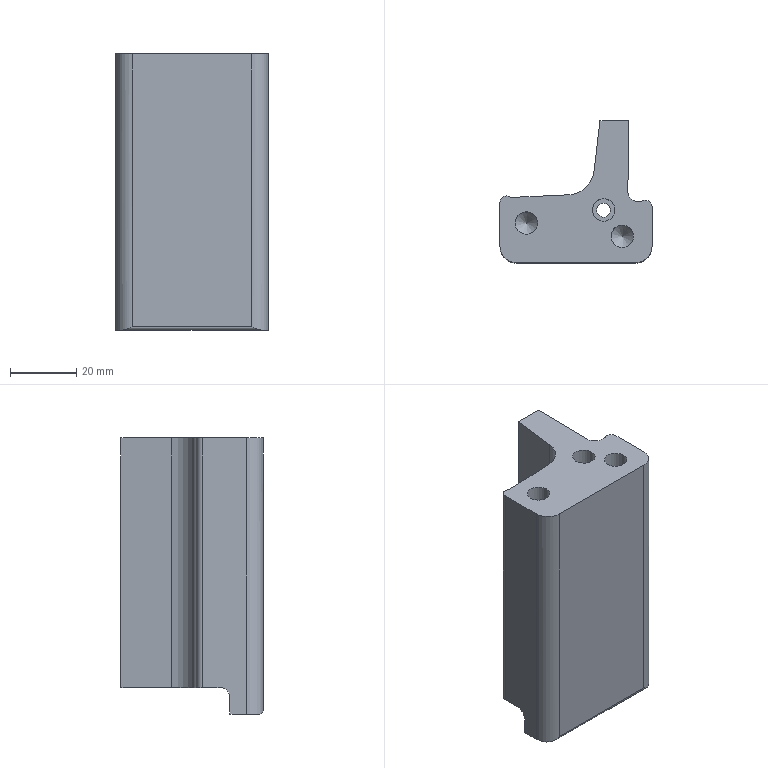Part | NX | features solid 2 | 1 solid | 32 faces | box 46 x 42.956 x 83.5 mm | volume 85744 mm3 | cylinder 15 | plane 14 | cone 3 | commonest cylinder face diameters 4 x4 6.8 x3 6 x2 10 x2 2 x1 4.2 x1
STEP:
#1=CARTESIAN_POINT('',(81.,-103.,-13.5));
#2=VERTEX_POINT('',#1);
#3=CARTESIAN_POINT('',(79.,-107.,-13.5));
#4=VERTEX_POINT('',#3);
#5=CARTESIAN_POINT('',(76.,-103.,-13.5));
#6=DIRECTION('',(0.,0.,-1.));
#7=DIRECTION('',(-1.,0.,0.));
#8=AXIS2_PLACEMENT_3D('',#5,#6,#7);
#9=CIRCLE('',#8,5.);
#10=EDGE_CURVE('',#2,#4,#9,.T.);
#11=ORIENTED_EDGE('',*,*,#10,.T.);
#12=CARTESIAN_POINT('',(37.,-107.,-13.5));
#13=VERTEX_POINT('',#12);
#14=CARTESIAN_POINT('',(16.212,-107.,-13.5));
#15=DIRECTION('',(-1.,0.,0.));
#16=VECTOR('',#15,1000.);
#17=LINE('',#14,#16);
#18=EDGE_CURVE('',#4,#13,#17,.T.);
#19=ORIENTED_EDGE('',*,*,#18,.T.);
#20=CARTESIAN_POINT('',(35.,-103.,-13.5));
#21=VERTEX_POINT('',#20);
#22=CARTESIAN_POINT('',(40.,-103.,-13.5));
#23=DIRECTION('',(0.,0.,-1.));
#24=DIRECTION('',(-1.,0.,0.));
#25=AXIS2_PLACEMENT_3D('',#22,#23,#24);
#26=CIRCLE('',#25,5.);
#27=EDGE_CURVE('',#13,#21,#26,.T.);
#28=ORIENTED_EDGE('',*,*,#27,.T.);
#29=CARTESIAN_POINT('',(35.,-98.,-13.5));
#30=VERTEX_POINT('',#29);
#31=CARTESIAN_POINT('',(35.,-108.,-13.5));
#32=DIRECTION('',(0.,1.,0.));
#33=VECTOR('',#32,1000.);
#34=LINE('',#31,#33);
#35=EDGE_CURVE('',#21,#30,#34,.T.);
#36=ORIENTED_EDGE('',*,*,#35,.T.);
#37=CARTESIAN_POINT('',(81.,-98.,-13.5));
#38=VERTEX_POINT('',#37);
#39=CARTESIAN_POINT('',(16.212,-98.,-13.5));
#40=DIRECTION('',(-1.,0.,0.));
#41=VECTOR('',#40,1000.);
#42=LINE('',#39,#41);
#43=EDGE_CURVE('',#38,#30,#42,.T.);
#44=ORIENTED_EDGE('',*,*,#43,.F.);
#45=CARTESIAN_POINT('',(81.,-108.,-13.5));
#46=DIRECTION('',(0.,1.,0.));
#47=VECTOR('',#46,1000.);
#48=LINE('',#45,#47);
#49=EDGE_CURVE('',#2,#38,#48,.T.);
#50=ORIENTED_EDGE('',*,*,#49,.F.);
#51=EDGE_LOOP('',(#11,#19,#28,#36,#44,#50));
#52=FACE_BOUND('',#51,.T.);
#53=CARTESIAN_POINT('',(55.4,-103.,-13.5));
#54=VERTEX_POINT('',#53);
#55=CARTESIAN_POINT('',(58.,-103.,-13.5));
#56=DIRECTION('',(0.,0.,-1.));
#57=DIRECTION('',(-1.,0.,0.));
#58=AXIS2_PLACEMENT_3D('',#55,#56,#57);
#59=CIRCLE('',#58,2.6);
#60=EDGE_CURVE('',#54,#54,#59,.F.);
#61=ORIENTED_EDGE('',*,*,#60,.T.);
#62=EDGE_LOOP('',(#61));
#63=FACE_BOUND('',#62,.T.);
#64=CARTESIAN_POINT('',(16.212,-108.,-13.5));
#65=DIRECTION('',(0.,0.,-1.));
#66=DIRECTION('',(-1.,0.,0.));
#67=AXIS2_PLACEMENT_3D('',#64,#65,#66);
#68=PLANE('',#67);
#69=ADVANCED_FACE('',(#52,#63),#68,.T.);
#70=CARTESIAN_POINT('',(46.4,-96.,70.));
#71=VERTEX_POINT('',#70);
#72=CARTESIAN_POINT('',(43.,-96.,70.));
#73=DIRECTION('',(0.,0.,-1.));
#74=DIRECTION('',(1.,0.,0.));
#75=AXIS2_PLACEMENT_3D('',#72,#73,#74);
#76=CIRCLE('',#75,3.4);
#77=EDGE_CURVE('',#71,#71,#76,.T.);
#78=ORIENTED_EDGE('',*,*,#77,.T.);
#79=EDGE_LOOP('',(#78));
#80=FACE_BOUND('',#79,.T.);
#81=CARTESIAN_POINT('',(69.763,-92.,70.));
#82=VERTEX_POINT('',#81);
#83=CARTESIAN_POINT('',(66.363,-92.,70.));
#84=DIRECTION('',(0.,0.,1.));
#85=DIRECTION('',(1.,0.,0.));
#86=AXIS2_PLACEMENT_3D('',#83,#84,#85);
#87=CIRCLE('',#86,3.4);
#88=EDGE_CURVE('',#82,#82,#87,.T.);
#89=ORIENTED_EDGE('',*,*,#88,.F.);
#90=EDGE_LOOP('',(#89));
#91=FACE_BOUND('',#90,.T.);
#92=CARTESIAN_POINT('',(73.954,-65.044,70.));
#93=VERTEX_POINT('',#92);
#94=CARTESIAN_POINT('',(73.682,-86.43,70.));
#95=VERTEX_POINT('',#94);
#96=CARTESIAN_POINT('',(74.016,-60.221,70.));
#97=DIRECTION('',(-0.01273,-0.9999,0.));
#98=VECTOR('',#97,1000.);
#99=LINE('',#96,#98);
#100=EDGE_CURVE('',#93,#95,#99,.T.);
#101=ORIENTED_EDGE('',*,*,#100,.F.);
#102=CARTESIAN_POINT('',(65.247,-65.044,70.));
#103=VERTEX_POINT('',#102);
#104=CARTESIAN_POINT('',(-37.5,-65.044,70.));
#105=DIRECTION('',(-1.,0.,0.));
#106=VECTOR('',#105,1000.);
#107=LINE('',#104,#106);
#108=EDGE_CURVE('',#103,#93,#107,.F.);
#109=ORIENTED_EDGE('',*,*,#108,.F.);
#110=CARTESIAN_POINT('',(63.441,-80.376,70.));
#111=VERTEX_POINT('',#110);
#112=CARTESIAN_POINT('',(63.441,-80.376,70.));
#113=DIRECTION('',(0.117,0.9931,0.));
#114=VECTOR('',#113,1000.);
#115=LINE('',#112,#114);
#116=EDGE_CURVE('',#103,#111,#115,.F.);
#117=ORIENTED_EDGE('',*,*,#116,.T.);
#118=CARTESIAN_POINT('',(55.874,-87.431,70.));
#119=VERTEX_POINT('',#118);
#120=CARTESIAN_POINT('',(55.496,-79.44,70.));
#121=DIRECTION('',(0.,0.,1.));
#122=DIRECTION('',(1.,0.,0.));
#123=AXIS2_PLACEMENT_3D('',#120,#121,#122);
#124=CIRCLE('',#123,8.);
#125=EDGE_CURVE('',#111,#119,#124,.F.);
#126=ORIENTED_EDGE('',*,*,#125,.T.);
#127=CARTESIAN_POINT('',(46.55,-87.872,70.));
#128=VERTEX_POINT('',#127);
#129=CARTESIAN_POINT('',(46.55,-87.872,70.));
#130=DIRECTION('',(0.9989,0.04722,0.));
#131=VECTOR('',#130,1000.);
#132=LINE('',#129,#131);
#133=EDGE_CURVE('',#119,#128,#132,.F.);
#134=ORIENTED_EDGE('',*,*,#133,.T.);
#135=CARTESIAN_POINT('',(38.87,-88.202,70.));
#136=VERTEX_POINT('',#135);
#137=CARTESIAN_POINT('',(38.87,-88.202,70.));
#138=DIRECTION('',(0.9991,0.0429,0.));
#139=VECTOR('',#138,1000.);
#140=LINE('',#137,#139);
#141=EDGE_CURVE('',#136,#128,#140,.T.);
#142=ORIENTED_EDGE('',*,*,#141,.F.);
#143=CARTESIAN_POINT('',(37.892,-87.994,70.));
#144=VERTEX_POINT('',#143);
#145=CARTESIAN_POINT('',(38.784,-86.203,70.));
#146=DIRECTION('',(0.,0.,1.));
#147=DIRECTION('',(1.,0.,0.));
#148=AXIS2_PLACEMENT_3D('',#145,#146,#147);
#149=CIRCLE('',#148,2.);
#150=EDGE_CURVE('',#144,#136,#149,.T.);
#151=ORIENTED_EDGE('',*,*,#150,.F.);
#152=CARTESIAN_POINT('',(35.,-89.784,70.));
#153=VERTEX_POINT('',#152);
#154=CARTESIAN_POINT('',(37.,-89.784,70.));
#155=DIRECTION('',(0.,0.,1.));
#156=DIRECTION('',(1.,0.,0.));
#157=AXIS2_PLACEMENT_3D('',#154,#155,#156);
#158=CIRCLE('',#157,2.);
#159=EDGE_CURVE('',#153,#144,#158,.F.);
#160=ORIENTED_EDGE('',*,*,#159,.F.);
#161=CARTESIAN_POINT('',(35.,-103.,70.));
#162=VERTEX_POINT('',#161);
#163=CARTESIAN_POINT('',(35.,-110.403,70.));
#164=DIRECTION('',(0.,1.,0.));
#165=VECTOR('',#164,1000.);
#166=LINE('',#163,#165);
#167=EDGE_CURVE('',#162,#153,#166,.T.);
#168=ORIENTED_EDGE('',*,*,#167,.F.);
#169=CARTESIAN_POINT('',(40.,-108.,70.));
#170=VERTEX_POINT('',#169);
#171=CARTESIAN_POINT('',(40.,-103.,70.));
#172=DIRECTION('',(0.,0.,1.));
#173=DIRECTION('',(1.,0.,0.));
#174=AXIS2_PLACEMENT_3D('',#171,#172,#173);
#175=CIRCLE('',#174,5.);
#176=EDGE_CURVE('',#170,#162,#175,.F.);
#177=ORIENTED_EDGE('',*,*,#176,.F.);
#178=CARTESIAN_POINT('',(76.,-108.,70.));
#179=VERTEX_POINT('',#178);
#180=CARTESIAN_POINT('',(16.212,-108.,70.));
#181=DIRECTION('',(-1.,0.,0.));
#182=VECTOR('',#181,1000.);
#183=LINE('',#180,#182);
#184=EDGE_CURVE('',#179,#170,#183,.T.);
#185=ORIENTED_EDGE('',*,*,#184,.F.);
#186=CARTESIAN_POINT('',(81.,-103.,70.));
#187=VERTEX_POINT('',#186);
#188=CARTESIAN_POINT('',(76.,-103.,70.));
#189=DIRECTION('',(0.,0.,1.));
#190=DIRECTION('',(1.,0.,0.));
#191=AXIS2_PLACEMENT_3D('',#188,#189,#190);
#192=CIRCLE('',#191,5.);
#193=EDGE_CURVE('',#187,#179,#192,.F.);
#194=ORIENTED_EDGE('',*,*,#193,.F.);
#195=CARTESIAN_POINT('',(81.,-91.098,70.));
#196=VERTEX_POINT('',#195);
#197=CARTESIAN_POINT('',(81.,-91.098,70.));
#198=DIRECTION('',(0.,-1.,0.));
#199=VECTOR('',#198,1000.);
#200=LINE('',#197,#199);
#201=EDGE_CURVE('',#196,#187,#200,.T.);
#202=ORIENTED_EDGE('',*,*,#201,.F.);
#203=CARTESIAN_POINT('',(78.127,-89.299,70.));
#204=VERTEX_POINT('',#203);
#205=CARTESIAN_POINT('',(79.,-91.098,70.));
#206=DIRECTION('',(0.,0.,1.));
#207=DIRECTION('',(1.,0.,0.));
#208=AXIS2_PLACEMENT_3D('',#205,#206,#207);
#209=CIRCLE('',#208,2.);
#210=EDGE_CURVE('',#204,#196,#209,.F.);
#211=ORIENTED_EDGE('',*,*,#210,.F.);
#212=CARTESIAN_POINT('',(77.147,-89.497,70.));
#213=VERTEX_POINT('',#212);
#214=CARTESIAN_POINT('',(77.253,-87.5,70.));
#215=DIRECTION('',(0.,0.,1.));
#216=DIRECTION('',(1.,0.,0.));
#217=AXIS2_PLACEMENT_3D('',#214,#215,#216);
#218=CIRCLE('',#217,2.);
#219=EDGE_CURVE('',#213,#204,#218,.T.);
#220=ORIENTED_EDGE('',*,*,#219,.F.);
#221=CARTESIAN_POINT('',(76.523,-89.464,70.));
#222=VERTEX_POINT('',#221);
#223=CARTESIAN_POINT('',(76.523,-89.464,70.));
#224=DIRECTION('',(0.9986,-0.05307,0.));
#225=VECTOR('',#224,1000.);
#226=LINE('',#223,#225);
#227=EDGE_CURVE('',#222,#213,#226,.T.);
#228=ORIENTED_EDGE('',*,*,#227,.F.);
#229=CARTESIAN_POINT('',(76.682,-86.468,70.));
#230=DIRECTION('',(0.,0.,1.));
#231=DIRECTION('',(1.,0.,0.));
#232=AXIS2_PLACEMENT_3D('',#229,#230,#231);
#233=CIRCLE('',#232,3.);
#234=EDGE_CURVE('',#95,#222,#233,.T.);
#235=ORIENTED_EDGE('',*,*,#234,.F.);
#236=EDGE_LOOP('',(#101,#109,#117,#126,#134,#142,#151,#160,#168,#177,#185,#194,#202,#211,#220,#228,#235));
#237=FACE_BOUND('',#236,.T.);
#238=CARTESIAN_POINT('',(75.4,-100.,70.));
#239=VERTEX_POINT('',#238);
#240=CARTESIAN_POINT('',(72.,-100.,70.));
#241=DIRECTION('',(0.,0.,-1.));
#242=DIRECTION('',(1.,0.,0.));
#243=AXIS2_PLACEMENT_3D('',#240,#241,#242);
#244=CIRCLE('',#243,3.4);
#245=EDGE_CURVE('',#239,#239,#244,.T.);
#246=ORIENTED_EDGE('',*,*,#245,.T.);
#247=EDGE_LOOP('',(#246));
#248=FACE_BOUND('',#247,.T.);
#249=CARTESIAN_POINT('',(-37.5,0.,70.));
#250=DIRECTION('',(0.,0.,1.));
#251=DIRECTION('',(1.,0.,0.));
#252=AXIS2_PLACEMENT_3D('',#249,#250,#251);
#253=PLANE('',#252);
#254=ADVANCED_FACE('',(#80,#91,#237,#248),#253,.T.);
#255=CARTESIAN_POINT('',(76.,-108.,-12.5));
#256=VERTEX_POINT('',#255);
#257=CARTESIAN_POINT('',(79.,-107.,-13.5));
#258=CARTESIAN_POINT('',(78.085,-107.686,-13.5));
#259=CARTESIAN_POINT('',(77.03,-108.,-12.961));
#260=CARTESIAN_POINT('',(76.,-108.,-12.5));
#261=B_SPLINE_CURVE_WITH_KNOTS('',3,(#257,#258,#259,#260),.UNSPECIFIED.,.F.,.F.,(4,4),(0.,0.003386),.UNSPECIFIED.);
#262=EDGE_CURVE('',#256,#4,#261,.F.);
#263=ORIENTED_EDGE('',*,*,#262,.F.);
#264=CARTESIAN_POINT('',(40.,-108.,-12.5));
#265=VERTEX_POINT('',#264);
#266=CARTESIAN_POINT('',(16.212,-108.,-12.5));
#267=DIRECTION('',(-1.,0.,0.));
#268=VECTOR('',#267,1000.);
#269=LINE('',#266,#268);
#270=EDGE_CURVE('',#265,#256,#269,.F.);
#271=ORIENTED_EDGE('',*,*,#270,.F.);
#272=CARTESIAN_POINT('',(37.,-107.,-13.5));
#273=CARTESIAN_POINT('',(37.915,-107.686,-13.5));
#274=CARTESIAN_POINT('',(38.97,-108.,-12.961));
#275=CARTESIAN_POINT('',(40.,-108.,-12.5));
#276=B_SPLINE_CURVE_WITH_KNOTS('',3,(#272,#273,#274,#275),.UNSPECIFIED.,.F.,.F.,(4,4),(0.,0.003386),.UNSPECIFIED.);
#277=EDGE_CURVE('',#13,#265,#276,.T.);
#278=ORIENTED_EDGE('',*,*,#277,.F.);
#279=ORIENTED_EDGE('',*,*,#18,.F.);
#280=EDGE_LOOP('',(#263,#271,#278,#279));
#281=FACE_BOUND('',#280,.T.);
#282=CARTESIAN_POINT('',(16.212,-107.,-12.5));
#283=DIRECTION('',(-1.,0.,0.));
#284=DIRECTION('',(0.,0.,1.));
#285=AXIS2_PLACEMENT_3D('',#282,#283,#284);
#286=CYLINDRICAL_SURFACE('',#285,1.);
#287=ADVANCED_FACE('',(#281),#286,.T.);
#288=CARTESIAN_POINT('',(35.,-98.,-8.5));
#289=VERTEX_POINT('',#288);
#290=CARTESIAN_POINT('',(35.,-98.,40.));
#291=DIRECTION('',(0.,0.,-1.));
#292=VECTOR('',#291,1000.);
#293=LINE('',#290,#292);
#294=EDGE_CURVE('',#289,#30,#293,.T.);
#295=ORIENTED_EDGE('',*,*,#294,.F.);
#296=CARTESIAN_POINT('',(81.,-98.,-8.5));
#297=VERTEX_POINT('',#296);
#298=CARTESIAN_POINT('',(81.,-98.,-8.5));
#299=DIRECTION('',(-1.,0.,0.));
#300=VECTOR('',#299,1000.);
#301=LINE('',#298,#300);
#302=EDGE_CURVE('',#289,#297,#301,.F.);
#303=ORIENTED_EDGE('',*,*,#302,.T.);
#304=CARTESIAN_POINT('',(81.,-98.,40.));
#305=DIRECTION('',(0.,0.,-1.));
#306=VECTOR('',#305,1000.);
#307=LINE('',#304,#306);
#308=EDGE_CURVE('',#297,#38,#307,.T.);
#309=ORIENTED_EDGE('',*,*,#308,.T.);
#310=ORIENTED_EDGE('',*,*,#43,.T.);
#311=EDGE_LOOP('',(#295,#303,#309,#310));
#312=FACE_BOUND('',#311,.T.);
#313=CARTESIAN_POINT('',(16.212,-98.,40.));
#314=DIRECTION('',(0.,-1.,0.));
#315=DIRECTION('',(0.,0.,-1.));
#316=AXIS2_PLACEMENT_3D('',#313,#314,#315);
#317=PLANE('',#316);
#318=ADVANCED_FACE('',(#312),#317,.F.);
#319=CARTESIAN_POINT('',(64.263,-92.,29.5));
#320=VERTEX_POINT('',#319);
#321=CARTESIAN_POINT('',(66.363,-92.,29.5));
#322=DIRECTION('',(0.,0.,-1.));
#323=DIRECTION('',(-1.,0.,0.));
#324=AXIS2_PLACEMENT_3D('',#321,#322,#323);
#325=CIRCLE('',#324,2.1);
#326=EDGE_CURVE('',#320,#320,#325,.T.);
#327=ORIENTED_EDGE('',*,*,#326,.T.);
#328=EDGE_LOOP('',(#327));
#329=FACE_BOUND('',#328,.T.);
#330=CARTESIAN_POINT('',(69.763,-92.,29.5));
#331=VERTEX_POINT('',#330);
#332=CARTESIAN_POINT('',(66.363,-92.,29.5));
#333=DIRECTION('',(0.,0.,1.));
#334=DIRECTION('',(1.,0.,0.));
#335=AXIS2_PLACEMENT_3D('',#332,#333,#334);
#336=CIRCLE('',#335,3.4);
#337=EDGE_CURVE('',#331,#331,#336,.F.);
#338=ORIENTED_EDGE('',*,*,#337,.F.);
#339=EDGE_LOOP('',(#338));
#340=FACE_BOUND('',#339,.T.);
#341=CARTESIAN_POINT('',(66.363,-92.,29.5));
#342=DIRECTION('',(0.,0.,-1.));
#343=DIRECTION('',(-1.,0.,0.));
#344=AXIS2_PLACEMENT_3D('',#341,#342,#343);
#345=PLANE('',#344);
#346=ADVANCED_FACE('',(#329,#340),#345,.F.);
#347=CARTESIAN_POINT('',(81.,-95.,-5.5));
#348=VERTEX_POINT('',#347);
#349=CARTESIAN_POINT('',(81.,-95.,-8.5));
#350=DIRECTION('',(1.,0.,0.));
#351=DIRECTION('',(0.,0.,-1.));
#352=AXIS2_PLACEMENT_3D('',#349,#350,#351);
#353=CIRCLE('',#352,3.);
#354=EDGE_CURVE('',#297,#348,#353,.F.);
#355=ORIENTED_EDGE('',*,*,#354,.F.);
#356=ORIENTED_EDGE('',*,*,#302,.F.);
#357=CARTESIAN_POINT('',(35.,-95.,-5.5));
#358=VERTEX_POINT('',#357);
#359=CARTESIAN_POINT('',(35.,-95.,-8.5));
#360=DIRECTION('',(-1.,0.,0.));
#361=DIRECTION('',(0.,-1.,0.));
#362=AXIS2_PLACEMENT_3D('',#359,#360,#361);
#363=CIRCLE('',#362,3.);
#364=EDGE_CURVE('',#358,#289,#363,.F.);
#365=ORIENTED_EDGE('',*,*,#364,.F.);
#366=CARTESIAN_POINT('',(35.,-95.,-5.5));
#367=DIRECTION('',(-1.,0.,0.));
#368=VECTOR('',#367,1000.);
#369=LINE('',#366,#368);
#370=EDGE_CURVE('',#348,#358,#369,.T.);
#371=ORIENTED_EDGE('',*,*,#370,.F.);
#372=EDGE_LOOP('',(#355,#356,#365,#371));
#373=FACE_BOUND('',#372,.T.);
#374=CARTESIAN_POINT('',(40.003,-95.,-8.5));
#375=DIRECTION('',(1.,0.,0.));
#376=DIRECTION('',(0.,0.,-1.));
#377=AXIS2_PLACEMENT_3D('',#374,#375,#376);
#378=CYLINDRICAL_SURFACE('',#377,3.);
#379=ADVANCED_FACE('',(#373),#378,.F.);
#380=ORIENTED_EDGE('',*,*,#326,.F.);
#381=EDGE_LOOP('',(#380));
#382=FACE_BOUND('',#381,.T.);
#383=CARTESIAN_POINT('',(68.463,-92.,-5.5));
#384=VERTEX_POINT('',#383);
#385=CARTESIAN_POINT('',(66.363,-92.,-5.5));
#386=DIRECTION('',(0.,0.,1.));
#387=DIRECTION('',(1.,0.,0.));
#388=AXIS2_PLACEMENT_3D('',#385,#386,#387);
#389=CIRCLE('',#388,2.1);
#390=EDGE_CURVE('',#384,#384,#389,.T.);
#391=ORIENTED_EDGE('',*,*,#390,.F.);
#392=EDGE_LOOP('',(#391));
#393=FACE_BOUND('',#392,.T.);
#394=CARTESIAN_POINT('',(66.363,-92.,32.5));
#395=DIRECTION('',(0.,0.,-1.));
#396=DIRECTION('',(1.,0.,0.));
#397=AXIS2_PLACEMENT_3D('',#394,#395,#396);
#398=CYLINDRICAL_SURFACE('',#397,2.1);
#399=ADVANCED_FACE('',(#382,#393),#398,.F.);
#400=CARTESIAN_POINT('',(73.682,-86.43,-5.5));
#401=VERTEX_POINT('',#400);
#402=CARTESIAN_POINT('',(73.682,-86.43,40.));
#403=DIRECTION('',(0.,0.,-1.));
#404=VECTOR('',#403,1000.);
#405=LINE('',#402,#404);
#406=EDGE_CURVE('',#95,#401,#405,.T.);
#407=ORIENTED_EDGE('',*,*,#406,.F.);
#408=ORIENTED_EDGE('',*,*,#234,.T.);
#409=CARTESIAN_POINT('',(76.523,-89.464,-5.5));
#410=VERTEX_POINT('',#409);
#411=CARTESIAN_POINT('',(76.523,-89.464,40.));
#412=DIRECTION('',(0.,0.,-1.));
#413=VECTOR('',#412,1000.);
#414=LINE('',#411,#413);
#415=EDGE_CURVE('',#222,#410,#414,.T.);
#416=ORIENTED_EDGE('',*,*,#415,.T.);
#417=CARTESIAN_POINT('',(76.682,-86.468,-5.5));
#418=DIRECTION('',(0.,0.,1.));
#419=DIRECTION('',(1.,0.,0.));
#420=AXIS2_PLACEMENT_3D('',#417,#418,#419);
#421=CIRCLE('',#420,3.);
#422=EDGE_CURVE('',#401,#410,#421,.T.);
#423=ORIENTED_EDGE('',*,*,#422,.F.);
#424=EDGE_LOOP('',(#407,#408,#416,#423));
#425=FACE_BOUND('',#424,.T.);
#426=CARTESIAN_POINT('',(76.682,-86.468,40.));
#427=DIRECTION('',(0.,0.,-1.));
#428=DIRECTION('',(-1.,0.,0.));
#429=AXIS2_PLACEMENT_3D('',#426,#427,#428);
#430=CYLINDRICAL_SURFACE('',#429,3.);
#431=ADVANCED_FACE('',(#425),#430,.F.);
#432=ORIENTED_EDGE('',*,*,#415,.F.);
#433=ORIENTED_EDGE('',*,*,#227,.T.);
#434=CARTESIAN_POINT('',(77.147,-89.497,-5.5));
#435=VERTEX_POINT('',#434);
#436=CARTESIAN_POINT('',(77.147,-89.497,40.));
#437=DIRECTION('',(0.,0.,-1.));
#438=VECTOR('',#437,1000.);
#439=LINE('',#436,#438);
#440=EDGE_CURVE('',#213,#435,#439,.T.);
#441=ORIENTED_EDGE('',*,*,#440,.T.);
#442=CARTESIAN_POINT('',(76.523,-89.464,-5.5));
#443=DIRECTION('',(0.9986,-0.05307,0.));
#444=VECTOR('',#443,1000.);
#445=LINE('',#442,#444);
#446=EDGE_CURVE('',#410,#435,#445,.T.);
#447=ORIENTED_EDGE('',*,*,#446,.F.);
#448=EDGE_LOOP('',(#432,#433,#441,#447));
#449=FACE_BOUND('',#448,.T.);
#450=CARTESIAN_POINT('',(76.523,-89.464,40.));
#451=DIRECTION('',(0.05307,0.9986,0.));
#452=DIRECTION('',(-0.9986,0.05307,0.));
#453=AXIS2_PLACEMENT_3D('',#450,#451,#452);
#454=PLANE('',#453);
#455=ADVANCED_FACE('',(#449),#454,.T.);
#456=ORIENTED_EDGE('',*,*,#440,.F.);
#457=ORIENTED_EDGE('',*,*,#219,.T.);
#458=CARTESIAN_POINT('',(78.127,-89.299,-5.5));
#459=VERTEX_POINT('',#458);
#460=CARTESIAN_POINT('',(78.127,-89.299,40.));
#461=DIRECTION('',(0.,0.,-1.));
#462=VECTOR('',#461,1000.);
#463=LINE('',#460,#462);
#464=EDGE_CURVE('',#204,#459,#463,.T.);
#465=ORIENTED_EDGE('',*,*,#464,.T.);
#466=CARTESIAN_POINT('',(77.253,-87.5,-5.5));
#467=DIRECTION('',(0.,0.,1.));
#468=DIRECTION('',(1.,0.,0.));
#469=AXIS2_PLACEMENT_3D('',#466,#467,#468);
#470=CIRCLE('',#469,2.);
#471=EDGE_CURVE('',#435,#459,#470,.T.);
#472=ORIENTED_EDGE('',*,*,#471,.F.);
#473=EDGE_LOOP('',(#456,#457,#465,#472));
#474=FACE_BOUND('',#473,.T.);
#475=CARTESIAN_POINT('',(77.253,-87.5,40.));
#476=DIRECTION('',(0.,0.,-1.));
#477=DIRECTION('',(-1.,0.,0.));
#478=AXIS2_PLACEMENT_3D('',#475,#476,#477);
#479=CYLINDRICAL_SURFACE('',#478,2.);
#480=ADVANCED_FACE('',(#474),#479,.F.);
#481=ORIENTED_EDGE('',*,*,#464,.F.);
#482=ORIENTED_EDGE('',*,*,#210,.T.);
#483=CARTESIAN_POINT('',(81.,-91.098,-5.5));
#484=VERTEX_POINT('',#483);
#485=CARTESIAN_POINT('',(81.,-91.098,40.));
#486=DIRECTION('',(0.,0.,-1.));
#487=VECTOR('',#486,1000.);
#488=LINE('',#485,#487);
#489=EDGE_CURVE('',#196,#484,#488,.T.);
#490=ORIENTED_EDGE('',*,*,#489,.T.);
#491=CARTESIAN_POINT('',(79.,-91.098,-5.5));
#492=DIRECTION('',(0.,0.,-1.));
#493=DIRECTION('',(1.,0.,0.));
#494=AXIS2_PLACEMENT_3D('',#491,#492,#493);
#495=CIRCLE('',#494,2.);
#496=EDGE_CURVE('',#459,#484,#495,.T.);
#497=ORIENTED_EDGE('',*,*,#496,.F.);
#498=EDGE_LOOP('',(#481,#482,#490,#497));
#499=FACE_BOUND('',#498,.T.);
#500=CARTESIAN_POINT('',(79.,-91.098,40.));
#501=DIRECTION('',(0.,0.,-1.));
#502=DIRECTION('',(-1.,0.,0.));
#503=AXIS2_PLACEMENT_3D('',#500,#501,#502);
#504=CYLINDRICAL_SURFACE('',#503,2.);
#505=ADVANCED_FACE('',(#499),#504,.T.);
#506=ORIENTED_EDGE('',*,*,#489,.F.);
#507=ORIENTED_EDGE('',*,*,#201,.T.);
#508=CARTESIAN_POINT('',(81.,-103.,40.));
#509=DIRECTION('',(0.,0.,-1.));
#510=VECTOR('',#509,1000.);
#511=LINE('',#508,#510);
#512=EDGE_CURVE('',#187,#2,#511,.T.);
#513=ORIENTED_EDGE('',*,*,#512,.T.);
#514=ORIENTED_EDGE('',*,*,#49,.T.);
#515=ORIENTED_EDGE('',*,*,#308,.F.);
#516=ORIENTED_EDGE('',*,*,#354,.T.);
#517=CARTESIAN_POINT('',(81.,-91.098,-5.5));
#518=DIRECTION('',(0.,-1.,0.));
#519=VECTOR('',#518,1000.);
#520=LINE('',#517,#519);
#521=EDGE_CURVE('',#484,#348,#520,.T.);
#522=ORIENTED_EDGE('',*,*,#521,.F.);
#523=EDGE_LOOP('',(#506,#507,#513,#514,#515,#516,#522));
#524=FACE_BOUND('',#523,.T.);
#525=CARTESIAN_POINT('',(81.,-91.098,40.));
#526=DIRECTION('',(1.,0.,0.));
#527=DIRECTION('',(0.,0.,-1.));
#528=AXIS2_PLACEMENT_3D('',#525,#526,#527);
#529=PLANE('',#528);
#530=ADVANCED_FACE('',(#524),#529,.T.);
#531=ORIENTED_EDGE('',*,*,#512,.F.);
#532=ORIENTED_EDGE('',*,*,#193,.T.);
#533=CARTESIAN_POINT('',(76.,-108.,40.));
#534=DIRECTION('',(0.,0.,-1.));
#535=VECTOR('',#534,1000.);
#536=LINE('',#533,#535);
#537=EDGE_CURVE('',#256,#179,#536,.F.);
#538=ORIENTED_EDGE('',*,*,#537,.F.);
#539=ORIENTED_EDGE('',*,*,#262,.T.);
#540=ORIENTED_EDGE('',*,*,#10,.F.);
#541=EDGE_LOOP('',(#531,#532,#538,#539,#540));
#542=FACE_BOUND('',#541,.T.);
#543=CARTESIAN_POINT('',(76.,-103.,40.));
#544=DIRECTION('',(0.,0.,-1.));
#545=DIRECTION('',(-1.,0.,0.));
#546=AXIS2_PLACEMENT_3D('',#543,#544,#545);
#547=CYLINDRICAL_SURFACE('',#546,5.);
#548=ADVANCED_FACE('',(#542),#547,.T.);
#549=ORIENTED_EDGE('',*,*,#537,.T.);
#550=ORIENTED_EDGE('',*,*,#184,.T.);
#551=CARTESIAN_POINT('',(40.,-108.,-11.5));
#552=DIRECTION('',(0.,0.,-1.));
#553=VECTOR('',#552,1000.);
#554=LINE('',#551,#553);
#555=EDGE_CURVE('',#170,#265,#554,.T.);
#556=ORIENTED_EDGE('',*,*,#555,.T.);
#557=ORIENTED_EDGE('',*,*,#270,.T.);
#558=EDGE_LOOP('',(#549,#550,#556,#557));
#559=FACE_BOUND('',#558,.T.);
#560=CARTESIAN_POINT('',(16.212,-108.,40.));
#561=DIRECTION('',(0.,-1.,0.));
#562=DIRECTION('',(0.,0.,-1.));
#563=AXIS2_PLACEMENT_3D('',#560,#561,#562);
#564=PLANE('',#563);
#565=ADVANCED_FACE('',(#559),#564,.T.);
#566=ORIENTED_EDGE('',*,*,#555,.F.);
#567=ORIENTED_EDGE('',*,*,#176,.T.);
#568=CARTESIAN_POINT('',(35.,-103.,40.));
#569=DIRECTION('',(0.,0.,-1.));
#570=VECTOR('',#569,1000.);
#571=LINE('',#568,#570);
#572=EDGE_CURVE('',#21,#162,#571,.F.);
#573=ORIENTED_EDGE('',*,*,#572,.F.);
#574=ORIENTED_EDGE('',*,*,#27,.F.);
#575=ORIENTED_EDGE('',*,*,#277,.T.);
#576=EDGE_LOOP('',(#566,#567,#573,#574,#575));
#577=FACE_BOUND('',#576,.T.);
#578=CARTESIAN_POINT('',(40.,-103.,40.));
#579=DIRECTION('',(0.,0.,1.));
#580=DIRECTION('',(1.,0.,0.));
#581=AXIS2_PLACEMENT_3D('',#578,#579,#580);
#582=CYLINDRICAL_SURFACE('',#581,5.);
#583=ADVANCED_FACE('',(#577),#582,.T.);
#584=ORIENTED_EDGE('',*,*,#572,.T.);
#585=ORIENTED_EDGE('',*,*,#167,.T.);
#586=CARTESIAN_POINT('',(35.,-89.784,-5.5));
#587=VERTEX_POINT('',#586);
#588=CARTESIAN_POINT('',(35.,-89.784,40.));
#589=DIRECTION('',(0.,0.,-1.));
#590=VECTOR('',#589,1000.);
#591=LINE('',#588,#590);
#592=EDGE_CURVE('',#153,#587,#591,.T.);
#593=ORIENTED_EDGE('',*,*,#592,.T.);
#594=CARTESIAN_POINT('',(35.,-110.403,-5.5));
#595=DIRECTION('',(0.,1.,0.));
#596=VECTOR('',#595,1000.);
#597=LINE('',#594,#596);
#598=EDGE_CURVE('',#358,#587,#597,.T.);
#599=ORIENTED_EDGE('',*,*,#598,.F.);
#600=ORIENTED_EDGE('',*,*,#364,.T.);
#601=ORIENTED_EDGE('',*,*,#294,.T.);
#602=ORIENTED_EDGE('',*,*,#35,.F.);
#603=EDGE_LOOP('',(#584,#585,#593,#599,#600,#601,#602));
#604=FACE_BOUND('',#603,.T.);
#605=CARTESIAN_POINT('',(35.,-110.403,40.));
#606=DIRECTION('',(-1.,0.,0.));
#607=DIRECTION('',(0.,-1.,0.));
#608=AXIS2_PLACEMENT_3D('',#605,#606,#607);
#609=PLANE('',#608);
#610=ADVANCED_FACE('',(#604),#609,.T.);
#611=ORIENTED_EDGE('',*,*,#592,.F.);
#612=ORIENTED_EDGE('',*,*,#159,.T.);
#613=CARTESIAN_POINT('',(37.892,-87.994,-5.5));
#614=VERTEX_POINT('',#613);
#615=CARTESIAN_POINT('',(37.892,-87.994,40.));
#616=DIRECTION('',(0.,0.,-1.));
#617=VECTOR('',#616,1000.);
#618=LINE('',#615,#617);
#619=EDGE_CURVE('',#144,#614,#618,.T.);
#620=ORIENTED_EDGE('',*,*,#619,.T.);
#621=CARTESIAN_POINT('',(37.,-89.784,-5.5));
#622=DIRECTION('',(0.,0.,-1.));
#623=DIRECTION('',(1.,0.,0.));
#624=AXIS2_PLACEMENT_3D('',#621,#622,#623);
#625=CIRCLE('',#624,2.);
#626=EDGE_CURVE('',#587,#614,#625,.T.);
#627=ORIENTED_EDGE('',*,*,#626,.F.);
#628=EDGE_LOOP('',(#611,#612,#620,#627));
#629=FACE_BOUND('',#628,.T.);
#630=CARTESIAN_POINT('',(37.,-89.784,40.));
#631=DIRECTION('',(0.,0.,-1.));
#632=DIRECTION('',(-1.,0.,0.));
#633=AXIS2_PLACEMENT_3D('',#630,#631,#632);
#634=CYLINDRICAL_SURFACE('',#633,2.);
#635=ADVANCED_FACE('',(#629),#634,.T.);
#636=ORIENTED_EDGE('',*,*,#619,.F.);
#637=ORIENTED_EDGE('',*,*,#150,.T.);
#638=CARTESIAN_POINT('',(38.87,-88.202,-5.5));
#639=VERTEX_POINT('',#638);
#640=CARTESIAN_POINT('',(38.87,-88.202,40.));
#641=DIRECTION('',(0.,0.,-1.));
#642=VECTOR('',#641,1000.);
#643=LINE('',#640,#642);
#644=EDGE_CURVE('',#136,#639,#643,.T.);
#645=ORIENTED_EDGE('',*,*,#644,.T.);
#646=CARTESIAN_POINT('',(38.784,-86.203,-5.5));
#647=DIRECTION('',(0.,0.,1.));
#648=DIRECTION('',(1.,0.,0.));
#649=AXIS2_PLACEMENT_3D('',#646,#647,#648);
#650=CIRCLE('',#649,2.);
#651=EDGE_CURVE('',#614,#639,#650,.T.);
#652=ORIENTED_EDGE('',*,*,#651,.F.);
#653=EDGE_LOOP('',(#636,#637,#645,#652));
#654=FACE_BOUND('',#653,.T.);
#655=CARTESIAN_POINT('',(38.784,-86.203,40.));
#656=DIRECTION('',(0.,0.,-1.));
#657=DIRECTION('',(-1.,0.,0.));
#658=AXIS2_PLACEMENT_3D('',#655,#656,#657);
#659=CYLINDRICAL_SURFACE('',#658,2.);
#660=ADVANCED_FACE('',(#654),#659,.F.);
#661=ORIENTED_EDGE('',*,*,#141,.T.);
#662=CARTESIAN_POINT('',(46.55,-87.872,-5.5));
#663=VERTEX_POINT('',#662);
#664=CARTESIAN_POINT('',(46.55,-87.872,40.));
#665=DIRECTION('',(0.,0.,-1.));
#666=VECTOR('',#665,1000.);
#667=LINE('',#664,#666);
#668=EDGE_CURVE('',#128,#663,#667,.T.);
#669=ORIENTED_EDGE('',*,*,#668,.T.);
#670=CARTESIAN_POINT('',(38.87,-88.202,-5.5));
#671=DIRECTION('',(0.9991,0.0429,0.));
#672=VECTOR('',#671,1000.);
#673=LINE('',#670,#672);
#674=EDGE_CURVE('',#639,#663,#673,.T.);
#675=ORIENTED_EDGE('',*,*,#674,.F.);
#676=ORIENTED_EDGE('',*,*,#644,.F.);
#677=EDGE_LOOP('',(#661,#669,#675,#676));
#678=FACE_BOUND('',#677,.T.);
#679=CARTESIAN_POINT('',(38.87,-88.202,40.));
#680=DIRECTION('',(-0.0429,0.9991,0.));
#681=DIRECTION('',(-0.9991,-0.0429,0.));
#682=AXIS2_PLACEMENT_3D('',#679,#680,#681);
#683=PLANE('',#682);
#684=ADVANCED_FACE('',(#678),#683,.T.);
#685=ORIENTED_EDGE('',*,*,#133,.F.);
#686=CARTESIAN_POINT('',(55.874,-87.431,-5.5));
#687=VERTEX_POINT('',#686);
#688=CARTESIAN_POINT('',(55.874,-87.431,40.));
#689=DIRECTION('',(0.,0.,-1.));
#690=VECTOR('',#689,1000.);
#691=LINE('',#688,#690);
#692=EDGE_CURVE('',#119,#687,#691,.T.);
#693=ORIENTED_EDGE('',*,*,#692,.T.);
#694=CARTESIAN_POINT('',(46.55,-87.872,-5.5));
#695=DIRECTION('',(0.9989,0.04722,0.));
#696=VECTOR('',#695,1000.);
#697=LINE('',#694,#696);
#698=EDGE_CURVE('',#663,#687,#697,.T.);
#699=ORIENTED_EDGE('',*,*,#698,.F.);
#700=ORIENTED_EDGE('',*,*,#668,.F.);
#701=EDGE_LOOP('',(#685,#693,#699,#700));
#702=FACE_BOUND('',#701,.T.);
#703=CARTESIAN_POINT('',(46.55,-87.872,40.));
#704=DIRECTION('',(-0.04722,0.9989,0.));
#705=DIRECTION('',(-0.9989,-0.04722,0.));
#706=AXIS2_PLACEMENT_3D('',#703,#704,#705);
#707=PLANE('',#706);
#708=ADVANCED_FACE('',(#702),#707,.T.);
#709=ORIENTED_EDGE('',*,*,#125,.F.);
#710=CARTESIAN_POINT('',(63.441,-80.376,-5.5));
#711=VERTEX_POINT('',#710);
#712=CARTESIAN_POINT('',(63.441,-80.376,40.));
#713=DIRECTION('',(0.,0.,-1.));
#714=VECTOR('',#713,1000.);
#715=LINE('',#712,#714);
#716=EDGE_CURVE('',#111,#711,#715,.T.);
#717=ORIENTED_EDGE('',*,*,#716,.T.);
#718=CARTESIAN_POINT('',(55.496,-79.44,-5.5));
#719=DIRECTION('',(0.,0.,1.));
#720=DIRECTION('',(1.,0.,0.));
#721=AXIS2_PLACEMENT_3D('',#718,#719,#720);
#722=CIRCLE('',#721,8.);
#723=EDGE_CURVE('',#687,#711,#722,.T.);
#724=ORIENTED_EDGE('',*,*,#723,.F.);
#725=ORIENTED_EDGE('',*,*,#692,.F.);
#726=EDGE_LOOP('',(#709,#717,#724,#725));
#727=FACE_BOUND('',#726,.T.);
#728=CARTESIAN_POINT('',(55.496,-79.44,40.));
#729=DIRECTION('',(0.,0.,-1.));
#730=DIRECTION('',(-1.,0.,0.));
#731=AXIS2_PLACEMENT_3D('',#728,#729,#730);
#732=CYLINDRICAL_SURFACE('',#731,8.);
#733=ADVANCED_FACE('',(#727),#732,.F.);
#734=ORIENTED_EDGE('',*,*,#88,.T.);
#735=EDGE_LOOP('',(#734));
#736=FACE_BOUND('',#735,.T.);
#737=ORIENTED_EDGE('',*,*,#337,.T.);
#738=EDGE_LOOP('',(#737));
#739=FACE_BOUND('',#738,.T.);
#740=CARTESIAN_POINT('',(66.363,-92.,29.5));
#741=DIRECTION('',(0.,0.,1.));
#742=DIRECTION('',(1.,0.,0.));
#743=AXIS2_PLACEMENT_3D('',#740,#741,#742);
#744=CYLINDRICAL_SURFACE('',#743,3.4);
#745=ADVANCED_FACE('',(#736,#739),#744,.F.);
#746=ORIENTED_EDGE('',*,*,#390,.T.);
#747=EDGE_LOOP('',(#746));
#748=FACE_BOUND('',#747,.T.);
#749=CARTESIAN_POINT('',(65.247,-65.044,-5.5));
#750=VERTEX_POINT('',#749);
#751=CARTESIAN_POINT('',(63.441,-80.376,-5.5));
#752=DIRECTION('',(0.117,0.9931,0.));
#753=VECTOR('',#752,1000.);
#754=LINE('',#751,#753);
#755=EDGE_CURVE('',#711,#750,#754,.T.);
#756=ORIENTED_EDGE('',*,*,#755,.T.);
#757=CARTESIAN_POINT('',(73.954,-65.044,-5.5));
#758=VERTEX_POINT('',#757);
#759=CARTESIAN_POINT('',(40.003,-65.044,-5.5));
#760=DIRECTION('',(-1.,0.,0.));
#761=VECTOR('',#760,1000.);
#762=LINE('',#759,#761);
#763=EDGE_CURVE('',#750,#758,#762,.F.);
#764=ORIENTED_EDGE('',*,*,#763,.T.);
#765=CARTESIAN_POINT('',(74.016,-60.221,-5.5));
#766=DIRECTION('',(-0.01273,-0.9999,0.));
#767=VECTOR('',#766,1000.);
#768=LINE('',#765,#767);
#769=EDGE_CURVE('',#758,#401,#768,.T.);
#770=ORIENTED_EDGE('',*,*,#769,.T.);
#771=ORIENTED_EDGE('',*,*,#422,.T.);
#772=ORIENTED_EDGE('',*,*,#446,.T.);
#773=ORIENTED_EDGE('',*,*,#471,.T.);
#774=ORIENTED_EDGE('',*,*,#496,.T.);
#775=ORIENTED_EDGE('',*,*,#521,.T.);
#776=ORIENTED_EDGE('',*,*,#370,.T.);
#777=ORIENTED_EDGE('',*,*,#598,.T.);
#778=ORIENTED_EDGE('',*,*,#626,.T.);
#779=ORIENTED_EDGE('',*,*,#651,.T.);
#780=ORIENTED_EDGE('',*,*,#674,.T.);
#781=ORIENTED_EDGE('',*,*,#698,.T.);
#782=ORIENTED_EDGE('',*,*,#723,.T.);
#783=EDGE_LOOP('',(#756,#764,#770,#771,#772,#773,#774,#775,#776,#777,#778,#779,#780,#781,#782));
#784=FACE_BOUND('',#783,.T.);
#785=CARTESIAN_POINT('',(40.003,-37.982,-5.5));
#786=DIRECTION('',(0.,0.,1.));
#787=DIRECTION('',(1.,0.,0.));
#788=AXIS2_PLACEMENT_3D('',#785,#786,#787);
#789=PLANE('',#788);
#790=ADVANCED_FACE('',(#748,#784),#789,.F.);
#791=ORIENTED_EDGE('',*,*,#769,.F.);
#792=CARTESIAN_POINT('',(73.954,-65.044,40.));
#793=DIRECTION('',(0.,0.,1.));
#794=VECTOR('',#793,1000.);
#795=LINE('',#792,#794);
#796=EDGE_CURVE('',#93,#758,#795,.F.);
#797=ORIENTED_EDGE('',*,*,#796,.F.);
#798=ORIENTED_EDGE('',*,*,#100,.T.);
#799=ORIENTED_EDGE('',*,*,#406,.T.);
#800=EDGE_LOOP('',(#791,#797,#798,#799));
#801=FACE_BOUND('',#800,.T.);
#802=CARTESIAN_POINT('',(74.016,-60.221,40.));
#803=DIRECTION('',(0.9999,-0.01273,0.));
#804=DIRECTION('',(0.01273,0.9999,0.));
#805=AXIS2_PLACEMENT_3D('',#802,#803,#804);
#806=PLANE('',#805);
#807=ADVANCED_FACE('',(#801),#806,.T.);
#808=ORIENTED_EDGE('',*,*,#116,.F.);
#809=CARTESIAN_POINT('',(65.247,-65.044,40.));
#810=DIRECTION('',(0.,0.,-1.));
#811=VECTOR('',#810,1000.);
#812=LINE('',#809,#811);
#813=EDGE_CURVE('',#103,#750,#812,.T.);
#814=ORIENTED_EDGE('',*,*,#813,.T.);
#815=ORIENTED_EDGE('',*,*,#755,.F.);
#816=ORIENTED_EDGE('',*,*,#716,.F.);
#817=EDGE_LOOP('',(#808,#814,#815,#816));
#818=FACE_BOUND('',#817,.T.);
#819=CARTESIAN_POINT('',(63.441,-80.376,40.));
#820=DIRECTION('',(-0.9931,0.117,0.));
#821=DIRECTION('',(-0.117,-0.9931,0.));
#822=AXIS2_PLACEMENT_3D('',#819,#820,#821);
#823=PLANE('',#822);
#824=ADVANCED_FACE('',(#818),#823,.T.);
#825=ORIENTED_EDGE('',*,*,#796,.T.);
#826=ORIENTED_EDGE('',*,*,#763,.F.);
#827=ORIENTED_EDGE('',*,*,#813,.F.);
#828=ORIENTED_EDGE('',*,*,#108,.T.);
#829=EDGE_LOOP('',(#825,#826,#827,#828));
#830=FACE_BOUND('',#829,.T.);
#831=CARTESIAN_POINT('',(11.506,-65.044,0.));
#832=DIRECTION('',(0.,1.,0.));
#833=DIRECTION('',(0.,0.,1.));
#834=AXIS2_PLACEMENT_3D('',#831,#832,#833);
#835=PLANE('',#834);
#836=ADVANCED_FACE('',(#830),#835,.T.);
#837=CARTESIAN_POINT('',(39.6,-96.,44.4));
#838=VERTEX_POINT('',#837);
#839=CARTESIAN_POINT('',(43.,-96.,44.4));
#840=DIRECTION('',(0.,0.,-1.));
#841=DIRECTION('',(-1.,0.,0.));
#842=AXIS2_PLACEMENT_3D('',#839,#840,#841);
#843=CIRCLE('',#842,3.4);
#844=EDGE_CURVE('',#838,#838,#843,.T.);
#845=ORIENTED_EDGE('',*,*,#844,.T.);
#846=EDGE_LOOP('',(#845));
#847=FACE_BOUND('',#846,.T.);
#848=ORIENTED_EDGE('',*,*,#77,.F.);
#849=EDGE_LOOP('',(#848));
#850=FACE_BOUND('',#849,.T.);
#851=CARTESIAN_POINT('',(43.,-96.,70.));
#852=DIRECTION('',(0.,0.,-1.));
#853=DIRECTION('',(1.,0.,0.));
#854=AXIS2_PLACEMENT_3D('',#851,#852,#853);
#855=CYLINDRICAL_SURFACE('',#854,3.4);
#856=ADVANCED_FACE('',(#847,#850),#855,.F.);
#857=CARTESIAN_POINT('',(43.,-96.,41.));
#858=VERTEX_POINT('',#857);
#859=VERTEX_LOOP('',#858);
#860=FACE_BOUND('',#859,.T.);
#861=ORIENTED_EDGE('',*,*,#844,.F.);
#862=EDGE_LOOP('',(#861));
#863=FACE_BOUND('',#862,.T.);
#864=CARTESIAN_POINT('',(43.,-96.,44.4));
#865=DIRECTION('',(0.,0.,1.));
#866=DIRECTION('',(1.,0.,0.));
#867=AXIS2_PLACEMENT_3D('',#864,#865,#866);
#868=CONICAL_SURFACE('',#867,3.4,0.7854);
#869=ADVANCED_FACE('',(#860,#863),#868,.F.);
#870=CARTESIAN_POINT('',(68.6,-100.,44.4));
#871=VERTEX_POINT('',#870);
#872=CARTESIAN_POINT('',(72.,-100.,44.4));
#873=DIRECTION('',(0.,0.,-1.));
#874=DIRECTION('',(-1.,0.,0.));
#875=AXIS2_PLACEMENT_3D('',#872,#873,#874);
#876=CIRCLE('',#875,3.4);
#877=EDGE_CURVE('',#871,#871,#876,.T.);
#878=ORIENTED_EDGE('',*,*,#877,.T.);
#879=EDGE_LOOP('',(#878));
#880=FACE_BOUND('',#879,.T.);
#881=ORIENTED_EDGE('',*,*,#245,.F.);
#882=EDGE_LOOP('',(#881));
#883=FACE_BOUND('',#882,.T.);
#884=CARTESIAN_POINT('',(72.,-100.,70.));
#885=DIRECTION('',(0.,0.,-1.));
#886=DIRECTION('',(1.,0.,0.));
#887=AXIS2_PLACEMENT_3D('',#884,#885,#886);
#888=CYLINDRICAL_SURFACE('',#887,3.4);
#889=ADVANCED_FACE('',(#880,#883),#888,.F.);
#890=CARTESIAN_POINT('',(72.,-100.,41.));
#891=VERTEX_POINT('',#890);
#892=VERTEX_LOOP('',#891);
#893=FACE_BOUND('',#892,.T.);
#894=ORIENTED_EDGE('',*,*,#877,.F.);
#895=EDGE_LOOP('',(#894));
#896=FACE_BOUND('',#895,.T.);
#897=CARTESIAN_POINT('',(72.,-100.,44.4));
#898=DIRECTION('',(0.,0.,1.));
#899=DIRECTION('',(1.,0.,0.));
#900=AXIS2_PLACEMENT_3D('',#897,#898,#899);
#901=CONICAL_SURFACE('',#900,3.4,0.7854);
#902=ADVANCED_FACE('',(#893,#896),#901,.F.);
#903=CARTESIAN_POINT('',(55.4,-103.,7.9));
#904=VERTEX_POINT('',#903);
#905=CARTESIAN_POINT('',(58.,-103.,7.9));
#906=DIRECTION('',(0.,0.,-1.));
#907=DIRECTION('',(-1.,0.,0.));
#908=AXIS2_PLACEMENT_3D('',#905,#906,#907);
#909=CIRCLE('',#908,2.6);
#910=EDGE_CURVE('',#904,#904,#909,.F.);
#911=ORIENTED_EDGE('',*,*,#910,.T.);
#912=EDGE_LOOP('',(#911));
#913=FACE_BOUND('',#912,.T.);
#914=ORIENTED_EDGE('',*,*,#60,.F.);
#915=EDGE_LOOP('',(#914));
#916=FACE_BOUND('',#915,.T.);
#917=CARTESIAN_POINT('',(58.,-103.,-13.5));
#918=DIRECTION('',(0.,0.,1.));
#919=DIRECTION('',(1.,0.,0.));
#920=AXIS2_PLACEMENT_3D('',#917,#918,#919);
#921=CYLINDRICAL_SURFACE('',#920,2.6);
#922=ADVANCED_FACE('',(#913,#916),#921,.F.);
#923=CARTESIAN_POINT('',(58.,-103.,10.5));
#924=VERTEX_POINT('',#923);
#925=VERTEX_LOOP('',#924);
#926=FACE_BOUND('',#925,.T.);
#927=ORIENTED_EDGE('',*,*,#910,.F.);
#928=EDGE_LOOP('',(#927));
#929=FACE_BOUND('',#928,.T.);
#930=CARTESIAN_POINT('',(58.,-103.,7.901));
#931=DIRECTION('',(0.,0.,-1.));
#932=DIRECTION('',(-1.,0.,0.));
#933=AXIS2_PLACEMENT_3D('',#930,#931,#932);
#934=CONICAL_SURFACE('',#933,2.599,0.7854);
#935=ADVANCED_FACE('',(#926,#929),#934,.F.);
#936=CLOSED_SHELL('',(#69,#254,#287,#318,#346,#379,#399,#431,#455,#480,#505,#530,#548,#565,#583,#610,#635,#660,#684,#708,#733,#745,#790,#807,#824,#836,#856,#869,#889,#902,#922,#935));
#937=MANIFOLD_SOLID_BREP('',#936);
#938=(LENGTH_UNIT()NAMED_UNIT(*)SI_UNIT(.MILLI.,.METRE.));
#939=UNCERTAINTY_MEASURE_WITH_UNIT(LENGTH_MEASURE(0.0508),#938,'','');
#940=(NAMED_UNIT(*)PLANE_ANGLE_UNIT()SI_UNIT($,.RADIAN.));
#941=(NAMED_UNIT(*)SI_UNIT($,.STERADIAN.)SOLID_ANGLE_UNIT());
#942=(GEOMETRIC_REPRESENTATION_CONTEXT(3)GLOBAL_UNCERTAINTY_ASSIGNED_CONTEXT((#939))GLOBAL_UNIT_ASSIGNED_CONTEXT((#938,#940,#941))REPRESENTATION_CONTEXT('',''));
#943=ADVANCED_BREP_SHAPE_REPRESENTATION('',(#937),#942);